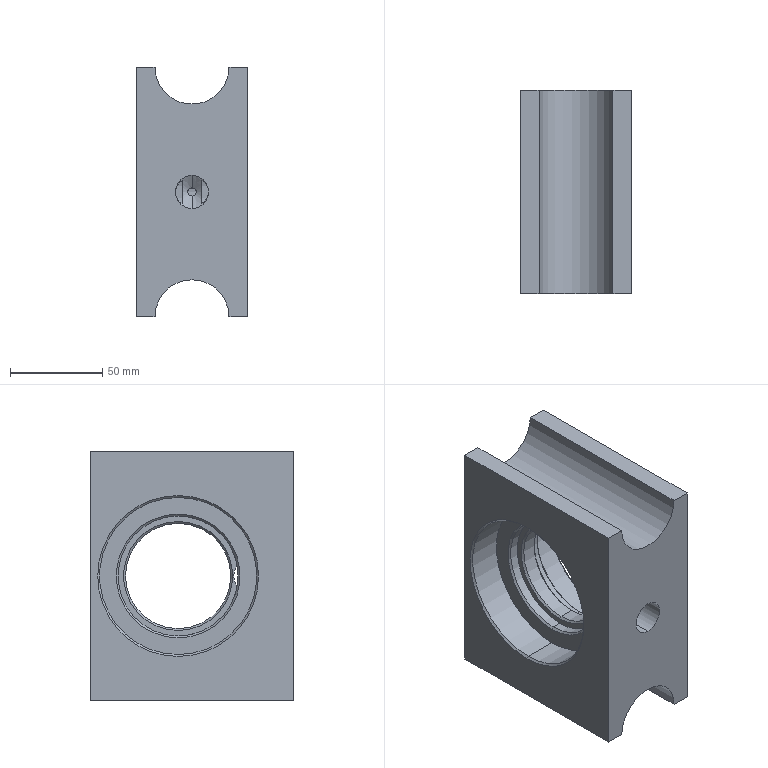Part | SolidWorks | features BaseBody 1 | 1 solid | 41 faces | box 60 x 110 x 135 mm | volume 463125 mm3 | cylinder 15 | cone 14 | plane 12 | commonest cylinder face diameters 65 x4 85 x4 40 x3 18 x2 57 x2
STEP:
#1=CARTESIAN_POINT('',(29.,7.5,42.5));
#2=VERTEX_POINT('',#1);
#3=CARTESIAN_POINT('',(29.,7.5,-42.5));
#4=VERTEX_POINT('',#3);
#5=CARTESIAN_POINT('',(29.,7.5,0.));
#6=DIRECTION('',(1.,0.,0.));
#7=DIRECTION('',(0.,0.,-1.));
#8=AXIS2_PLACEMENT_3D('',#5,#6,#7);
#9=CIRCLE('',#8,42.5);
#10=EDGE_CURVE('',#2,#4,#9,.T.);
#11=ORIENTED_EDGE('',*,*,#10,.F.);
#12=CARTESIAN_POINT('',(30.,7.5,43.5));
#13=VERTEX_POINT('',#12);
#14=CARTESIAN_POINT('',(29.,7.5,42.5));
#15=DIRECTION('',(0.7071,0.,0.7071));
#16=VECTOR('',#15,1000.);
#17=LINE('',#14,#16);
#18=EDGE_CURVE('',#2,#13,#17,.T.);
#19=ORIENTED_EDGE('',*,*,#18,.T.);
#20=CARTESIAN_POINT('',(30.,7.5,-43.5));
#21=VERTEX_POINT('',#20);
#22=CARTESIAN_POINT('',(30.,7.5,0.));
#23=DIRECTION('',(-1.,0.,0.));
#24=DIRECTION('',(0.,0.,-1.));
#25=AXIS2_PLACEMENT_3D('',#22,#23,#24);
#26=CIRCLE('',#25,43.5);
#27=EDGE_CURVE('',#21,#13,#26,.T.);
#28=ORIENTED_EDGE('',*,*,#27,.F.);
#29=CARTESIAN_POINT('',(29.,7.5,-42.5));
#30=DIRECTION('',(0.7071,0.,-0.7071));
#31=VECTOR('',#30,1000.);
#32=LINE('',#29,#31);
#33=EDGE_CURVE('',#4,#21,#32,.T.);
#34=ORIENTED_EDGE('',*,*,#33,.F.);
#35=EDGE_LOOP('',(#11,#19,#28,#34));
#36=FACE_OUTER_BOUND('',#35,.T.);
#37=CARTESIAN_POINT('',(29.,7.5,0.));
#38=DIRECTION('',(1.,0.,0.));
#39=DIRECTION('',(0.,0.,-1.));
#40=AXIS2_PLACEMENT_3D('',#37,#38,#39);
#41=CONICAL_SURFACE('',#40,42.5,0.7854);
#42=ADVANCED_FACE('',(#36),#41,.F.);
#43=CARTESIAN_POINT('',(10.,7.5,32.5));
#44=VERTEX_POINT('',#43);
#45=CARTESIAN_POINT('',(10.,7.5,-32.5));
#46=VERTEX_POINT('',#45);
#47=CARTESIAN_POINT('',(10.,7.5,0.));
#48=DIRECTION('',(1.,0.,0.));
#49=DIRECTION('',(0.,0.,-1.));
#50=AXIS2_PLACEMENT_3D('',#47,#48,#49);
#51=CIRCLE('',#50,32.5);
#52=EDGE_CURVE('',#44,#46,#51,.T.);
#53=ORIENTED_EDGE('',*,*,#52,.F.);
#54=CARTESIAN_POINT('',(11.,7.5,33.5));
#55=VERTEX_POINT('',#54);
#56=CARTESIAN_POINT('',(10.,7.5,32.5));
#57=DIRECTION('',(0.7071,0.,0.7071));
#58=VECTOR('',#57,1000.);
#59=LINE('',#56,#58);
#60=EDGE_CURVE('',#44,#55,#59,.T.);
#61=ORIENTED_EDGE('',*,*,#60,.T.);
#62=CARTESIAN_POINT('',(11.,7.5,-33.5));
#63=VERTEX_POINT('',#62);
#64=CARTESIAN_POINT('',(11.,7.5,0.));
#65=DIRECTION('',(-1.,0.,0.));
#66=DIRECTION('',(0.,0.,-1.));
#67=AXIS2_PLACEMENT_3D('',#64,#65,#66);
#68=CIRCLE('',#67,33.5);
#69=EDGE_CURVE('',#63,#55,#68,.T.);
#70=ORIENTED_EDGE('',*,*,#69,.F.);
#71=CARTESIAN_POINT('',(10.,7.5,-32.5));
#72=DIRECTION('',(0.7071,0.,-0.7071));
#73=VECTOR('',#72,1000.);
#74=LINE('',#71,#73);
#75=EDGE_CURVE('',#46,#63,#74,.T.);
#76=ORIENTED_EDGE('',*,*,#75,.F.);
#77=EDGE_LOOP('',(#53,#61,#70,#76));
#78=FACE_OUTER_BOUND('',#77,.T.);
#79=CARTESIAN_POINT('',(10.,7.5,0.));
#80=DIRECTION('',(1.,0.,0.));
#81=DIRECTION('',(0.,0.,-1.));
#82=AXIS2_PLACEMENT_3D('',#79,#80,#81);
#83=CONICAL_SURFACE('',#82,32.5,0.7854);
#84=ADVANCED_FACE('',(#78),#83,.F.);
#85=CARTESIAN_POINT('',(4.,7.5,28.5));
#86=VERTEX_POINT('',#85);
#87=CARTESIAN_POINT('',(4.,7.5,-28.5));
#88=VERTEX_POINT('',#87);
#89=CARTESIAN_POINT('',(4.,7.5,0.));
#90=DIRECTION('',(1.,0.,0.));
#91=DIRECTION('',(0.,0.,-1.));
#92=AXIS2_PLACEMENT_3D('',#89,#90,#91);
#93=CIRCLE('',#92,28.5);
#94=EDGE_CURVE('',#86,#88,#93,.T.);
#95=ORIENTED_EDGE('',*,*,#94,.F.);
#96=CARTESIAN_POINT('',(5.,7.5,29.5));
#97=VERTEX_POINT('',#96);
#98=CARTESIAN_POINT('',(4.,7.5,28.5));
#99=DIRECTION('',(0.7071,0.,0.7071));
#100=VECTOR('',#99,1000.);
#101=LINE('',#98,#100);
#102=EDGE_CURVE('',#86,#97,#101,.T.);
#103=ORIENTED_EDGE('',*,*,#102,.T.);
#104=CARTESIAN_POINT('',(5.,7.5,-29.5));
#105=VERTEX_POINT('',#104);
#106=CARTESIAN_POINT('',(5.,7.5,0.));
#107=DIRECTION('',(-1.,0.,0.));
#108=DIRECTION('',(0.,0.,-1.));
#109=AXIS2_PLACEMENT_3D('',#106,#107,#108);
#110=CIRCLE('',#109,29.5);
#111=EDGE_CURVE('',#105,#97,#110,.T.);
#112=ORIENTED_EDGE('',*,*,#111,.F.);
#113=CARTESIAN_POINT('',(4.,7.5,-28.5));
#114=DIRECTION('',(0.7071,0.,-0.7071));
#115=VECTOR('',#114,1000.);
#116=LINE('',#113,#115);
#117=EDGE_CURVE('',#88,#105,#116,.T.);
#118=ORIENTED_EDGE('',*,*,#117,.F.);
#119=EDGE_LOOP('',(#95,#103,#112,#118));
#120=FACE_OUTER_BOUND('',#119,.T.);
#121=CARTESIAN_POINT('',(4.,7.5,0.));
#122=DIRECTION('',(1.,0.,0.));
#123=DIRECTION('',(0.,0.,-1.));
#124=AXIS2_PLACEMENT_3D('',#121,#122,#123);
#125=CONICAL_SURFACE('',#124,28.5,0.7854);
#126=ADVANCED_FACE('',(#120),#125,.F.);
#127=CARTESIAN_POINT('',(-4.,7.5,-28.5));
#128=VERTEX_POINT('',#127);
#129=CARTESIAN_POINT('',(-4.,7.5,28.5));
#130=VERTEX_POINT('',#129);
#131=CARTESIAN_POINT('',(-4.,7.5,0.));
#132=DIRECTION('',(-1.,0.,0.));
#133=DIRECTION('',(0.,0.,1.));
#134=AXIS2_PLACEMENT_3D('',#131,#132,#133);
#135=CIRCLE('',#134,28.5);
#136=EDGE_CURVE('',#128,#130,#135,.T.);
#137=ORIENTED_EDGE('',*,*,#136,.F.);
#138=CARTESIAN_POINT('',(-5.,7.5,-29.5));
#139=VERTEX_POINT('',#138);
#140=CARTESIAN_POINT('',(-4.,7.5,-28.5));
#141=DIRECTION('',(-0.7071,0.,-0.7071));
#142=VECTOR('',#141,1000.);
#143=LINE('',#140,#142);
#144=EDGE_CURVE('',#128,#139,#143,.T.);
#145=ORIENTED_EDGE('',*,*,#144,.T.);
#146=CARTESIAN_POINT('',(-5.,7.5,29.5));
#147=VERTEX_POINT('',#146);
#148=CARTESIAN_POINT('',(-5.,7.5,0.));
#149=DIRECTION('',(1.,0.,0.));
#150=DIRECTION('',(0.,0.,1.));
#151=AXIS2_PLACEMENT_3D('',#148,#149,#150);
#152=CIRCLE('',#151,29.5);
#153=EDGE_CURVE('',#147,#139,#152,.T.);
#154=ORIENTED_EDGE('',*,*,#153,.F.);
#155=CARTESIAN_POINT('',(-4.,7.5,28.5));
#156=DIRECTION('',(-0.7071,0.,0.7071));
#157=VECTOR('',#156,1000.);
#158=LINE('',#155,#157);
#159=EDGE_CURVE('',#130,#147,#158,.T.);
#160=ORIENTED_EDGE('',*,*,#159,.F.);
#161=EDGE_LOOP('',(#137,#145,#154,#160));
#162=FACE_OUTER_BOUND('',#161,.T.);
#163=CARTESIAN_POINT('',(-4.,7.5,0.));
#164=DIRECTION('',(-1.,0.,0.));
#165=DIRECTION('',(0.,0.,1.));
#166=AXIS2_PLACEMENT_3D('',#163,#164,#165);
#167=CONICAL_SURFACE('',#166,28.5,0.7854);
#168=ADVANCED_FACE('',(#162),#167,.F.);
#169=CARTESIAN_POINT('',(-10.,7.5,-32.5));
#170=VERTEX_POINT('',#169);
#171=CARTESIAN_POINT('',(-10.,7.5,32.5));
#172=VERTEX_POINT('',#171);
#173=CARTESIAN_POINT('',(-10.,7.5,0.));
#174=DIRECTION('',(-1.,0.,0.));
#175=DIRECTION('',(0.,0.,1.));
#176=AXIS2_PLACEMENT_3D('',#173,#174,#175);
#177=CIRCLE('',#176,32.5);
#178=EDGE_CURVE('',#170,#172,#177,.T.);
#179=ORIENTED_EDGE('',*,*,#178,.F.);
#180=CARTESIAN_POINT('',(-11.,7.5,-33.5));
#181=VERTEX_POINT('',#180);
#182=CARTESIAN_POINT('',(-11.,7.5,-33.5));
#183=DIRECTION('',(-0.7071,0.,-0.7071));
#184=VECTOR('',#183,1000.);
#185=LINE('',#182,#184);
#186=EDGE_CURVE('',#170,#181,#185,.T.);
#187=ORIENTED_EDGE('',*,*,#186,.T.);
#188=CARTESIAN_POINT('',(-11.,7.5,33.5));
#189=VERTEX_POINT('',#188);
#190=CARTESIAN_POINT('',(-11.,7.5,0.));
#191=DIRECTION('',(1.,0.,0.));
#192=DIRECTION('',(0.,0.,1.));
#193=AXIS2_PLACEMENT_3D('',#190,#191,#192);
#194=CIRCLE('',#193,33.5);
#195=EDGE_CURVE('',#189,#181,#194,.T.);
#196=ORIENTED_EDGE('',*,*,#195,.F.);
#197=CARTESIAN_POINT('',(-11.,7.5,33.5));
#198=DIRECTION('',(-0.7071,0.,0.7071));
#199=VECTOR('',#198,1000.);
#200=LINE('',#197,#199);
#201=EDGE_CURVE('',#172,#189,#200,.T.);
#202=ORIENTED_EDGE('',*,*,#201,.F.);
#203=EDGE_LOOP('',(#179,#187,#196,#202));
#204=FACE_OUTER_BOUND('',#203,.T.);
#205=CARTESIAN_POINT('',(-11.,7.5,0.));
#206=DIRECTION('',(-1.,0.,0.));
#207=DIRECTION('',(0.,0.,1.));
#208=AXIS2_PLACEMENT_3D('',#205,#206,#207);
#209=CONICAL_SURFACE('',#208,33.5,0.7854);
#210=ADVANCED_FACE('',(#204),#209,.F.);
#211=CARTESIAN_POINT('',(-29.,7.5,-42.5));
#212=VERTEX_POINT('',#211);
#213=CARTESIAN_POINT('',(-29.,7.5,42.5));
#214=VERTEX_POINT('',#213);
#215=CARTESIAN_POINT('',(-29.,7.5,0.));
#216=DIRECTION('',(-1.,0.,0.));
#217=DIRECTION('',(0.,0.,-1.));
#218=AXIS2_PLACEMENT_3D('',#215,#216,#217);
#219=CIRCLE('',#218,42.5);
#220=EDGE_CURVE('',#212,#214,#219,.T.);
#221=ORIENTED_EDGE('',*,*,#220,.F.);
#222=CARTESIAN_POINT('',(-30.,7.5,-43.5));
#223=VERTEX_POINT('',#222);
#224=CARTESIAN_POINT('',(-30.,7.5,-43.5));
#225=DIRECTION('',(-0.7071,0.,-0.7071));
#226=VECTOR('',#225,1000.);
#227=LINE('',#224,#226);
#228=EDGE_CURVE('',#212,#223,#227,.T.);
#229=ORIENTED_EDGE('',*,*,#228,.T.);
#230=CARTESIAN_POINT('',(-30.,7.5,43.5));
#231=VERTEX_POINT('',#230);
#232=CARTESIAN_POINT('',(-30.,7.5,0.));
#233=DIRECTION('',(1.,0.,0.));
#234=DIRECTION('',(0.,0.,-1.));
#235=AXIS2_PLACEMENT_3D('',#232,#233,#234);
#236=CIRCLE('',#235,43.5);
#237=EDGE_CURVE('',#231,#223,#236,.T.);
#238=ORIENTED_EDGE('',*,*,#237,.F.);
#239=CARTESIAN_POINT('',(-30.,7.5,43.5));
#240=DIRECTION('',(-0.7071,0.,0.7071));
#241=VECTOR('',#240,1000.);
#242=LINE('',#239,#241);
#243=EDGE_CURVE('',#214,#231,#242,.T.);
#244=ORIENTED_EDGE('',*,*,#243,.F.);
#245=EDGE_LOOP('',(#221,#229,#238,#244));
#246=FACE_OUTER_BOUND('',#245,.T.);
#247=CARTESIAN_POINT('',(-30.,7.5,0.));
#248=DIRECTION('',(-1.,0.,0.));
#249=DIRECTION('',(0.,0.,1.));
#250=AXIS2_PLACEMENT_3D('',#247,#248,#249);
#251=CONICAL_SURFACE('',#250,43.5,0.7854);
#252=ADVANCED_FACE('',(#246),#251,.F.);
#253=CARTESIAN_POINT('',(-5.,-24.396,-6.238));
#254=VERTEX_POINT('',#253);
#255=CARTESIAN_POINT('',(-5.,7.5,-32.5));
#256=VERTEX_POINT('',#255);
#257=CARTESIAN_POINT('',(-5.,7.5,0.));
#258=DIRECTION('',(1.,0.,0.));
#259=DIRECTION('',(0.,0.,-1.));
#260=AXIS2_PLACEMENT_3D('',#257,#258,#259);
#261=CIRCLE('',#260,32.5);
#262=EDGE_CURVE('',#254,#256,#261,.T.);
#263=ORIENTED_EDGE('',*,*,#262,.T.);
#264=CARTESIAN_POINT('',(-5.,7.5,-32.5));
#265=DIRECTION('',(-1.,0.,0.));
#266=VECTOR('',#265,1000.);
#267=LINE('',#264,#266);
#268=EDGE_CURVE('',#256,#170,#267,.T.);
#269=ORIENTED_EDGE('',*,*,#268,.T.);
#270=ORIENTED_EDGE('',*,*,#178,.T.);
#271=CARTESIAN_POINT('',(-5.,7.5,32.5));
#272=VERTEX_POINT('',#271);
#273=CARTESIAN_POINT('',(-5.,7.5,32.5));
#274=DIRECTION('',(-1.,0.,0.));
#275=VECTOR('',#274,1000.);
#276=LINE('',#273,#275);
#277=EDGE_CURVE('',#272,#172,#276,.T.);
#278=ORIENTED_EDGE('',*,*,#277,.F.);
#279=CARTESIAN_POINT('',(-5.,-24.396,6.238));
#280=VERTEX_POINT('',#279);
#281=CARTESIAN_POINT('',(-5.,7.5,0.));
#282=DIRECTION('',(1.,0.,0.));
#283=DIRECTION('',(0.,0.,-1.));
#284=AXIS2_PLACEMENT_3D('',#281,#282,#283);
#285=CIRCLE('',#284,32.5);
#286=EDGE_CURVE('',#272,#280,#285,.T.);
#287=ORIENTED_EDGE('',*,*,#286,.T.);
#288=CARTESIAN_POINT('',(-9.,-25.,0.));
#289=VERTEX_POINT('',#288);
#290=CARTESIAN_POINT('',(-5.,-24.396,6.238));
#291=CARTESIAN_POINT('',(-5.564,-24.458,5.919));
#292=CARTESIAN_POINT('',(-6.087,-24.526,5.547));
#293=CARTESIAN_POINT('',(-6.808,-24.629,4.902));
#294=CARTESIAN_POINT('',(-7.038,-24.664,4.67));
#295=CARTESIAN_POINT('',(-7.467,-24.731,4.182));
#296=CARTESIAN_POINT('',(-7.664,-24.763,3.926));
#297=CARTESIAN_POINT('',(-8.025,-24.824,3.392));
#298=CARTESIAN_POINT('',(-8.188,-24.852,3.112));
#299=CARTESIAN_POINT('',(-8.476,-24.903,2.527));
#300=CARTESIAN_POINT('',(-8.599,-24.925,2.223));
#301=CARTESIAN_POINT('',(-8.796,-24.962,1.608));
#302=CARTESIAN_POINT('',(-8.872,-24.976,1.295));
#303=CARTESIAN_POINT('',(-8.973,-24.995,0.6557));
#304=CARTESIAN_POINT('',(-9.,-25.,0.3269));
#305=CARTESIAN_POINT('',(-9.,-25.,0.));
#306=B_SPLINE_CURVE_WITH_KNOTS('',3,(#290,#291,#292,#293,#294,#295,#296,#297,#298,#299,#300,#301,#302,#303,#304,#305),.UNSPECIFIED.,.F.,.F.,(4,2,2,2,2,2,2,4),(0.000451,0.002388,0.003357,0.004325,0.005294,0.006262,0.007231,0.008199),.UNSPECIFIED.);
#307=EDGE_CURVE('',#280,#289,#306,.T.);
#308=ORIENTED_EDGE('',*,*,#307,.T.);
#309=CARTESIAN_POINT('',(-9.,-25.,0.));
#310=CARTESIAN_POINT('',(-9.,-25.,-0.6513));
#311=CARTESIAN_POINT('',(-8.898,-24.98,-1.291));
#312=CARTESIAN_POINT('',(-8.499,-24.907,-2.535));
#313=CARTESIAN_POINT('',(-8.212,-24.855,-3.113));
#314=CARTESIAN_POINT('',(-7.485,-24.733,-4.193));
#315=CARTESIAN_POINT('',(-7.057,-24.665,-4.676));
#316=CARTESIAN_POINT('',(-6.336,-24.562,-5.325));
#317=CARTESIAN_POINT('',(-6.081,-24.527,-5.529));
#318=CARTESIAN_POINT('',(-5.555,-24.46,-5.905));
#319=CARTESIAN_POINT('',(-5.282,-24.427,-6.078));
#320=CARTESIAN_POINT('',(-5.,-24.396,-6.238));
#321=B_SPLINE_CURVE_WITH_KNOTS('',3,(#309,#310,#311,#312,#313,#314,#315,#316,#317,#318,#319,#320),.UNSPECIFIED.,.F.,.F.,(4,2,2,2,2,4),(0.008199,0.01013,0.01206,0.01399,0.01495,0.01592),.UNSPECIFIED.);
#322=EDGE_CURVE('',#289,#254,#321,.T.);
#323=ORIENTED_EDGE('',*,*,#322,.T.);
#324=EDGE_LOOP('',(#263,#269,#270,#278,#287,#308,#323));
#325=FACE_OUTER_BOUND('',#324,.T.);
#326=CARTESIAN_POINT('',(-5.,7.5,0.));
#327=DIRECTION('',(-1.,0.,0.));
#328=DIRECTION('',(0.,0.,1.));
#329=AXIS2_PLACEMENT_3D('',#326,#327,#328);
#330=CYLINDRICAL_SURFACE('',#329,32.5);
#331=ADVANCED_FACE('',(#325),#330,.F.);
#332=CARTESIAN_POINT('',(-11.,7.5,42.5));
#333=VERTEX_POINT('',#332);
#334=CARTESIAN_POINT('',(-11.,7.5,-42.5));
#335=VERTEX_POINT('',#334);
#336=CARTESIAN_POINT('',(-11.,7.5,0.));
#337=DIRECTION('',(1.,0.,0.));
#338=DIRECTION('',(0.,0.,-1.));
#339=AXIS2_PLACEMENT_3D('',#336,#337,#338);
#340=CIRCLE('',#339,42.5);
#341=EDGE_CURVE('',#333,#335,#340,.T.);
#342=ORIENTED_EDGE('',*,*,#341,.T.);
#343=CARTESIAN_POINT('',(-11.,7.5,-42.5));
#344=DIRECTION('',(-1.,0.,0.));
#345=VECTOR('',#344,1000.);
#346=LINE('',#343,#345);
#347=EDGE_CURVE('',#335,#212,#346,.T.);
#348=ORIENTED_EDGE('',*,*,#347,.T.);
#349=ORIENTED_EDGE('',*,*,#220,.T.);
#350=CARTESIAN_POINT('',(-11.,7.5,42.5));
#351=DIRECTION('',(-1.,0.,0.));
#352=VECTOR('',#351,1000.);
#353=LINE('',#350,#352);
#354=EDGE_CURVE('',#333,#214,#353,.T.);
#355=ORIENTED_EDGE('',*,*,#354,.F.);
#356=EDGE_LOOP('',(#342,#348,#349,#355));
#357=FACE_OUTER_BOUND('',#356,.T.);
#358=CARTESIAN_POINT('',(-11.,7.5,0.));
#359=DIRECTION('',(-1.,0.,0.));
#360=DIRECTION('',(0.,0.,1.));
#361=AXIS2_PLACEMENT_3D('',#358,#359,#360);
#362=CYLINDRICAL_SURFACE('',#361,42.5);
#363=ADVANCED_FACE('',(#357),#362,.F.);
#364=CARTESIAN_POINT('',(0.,-25.,9.));
#365=VERTEX_POINT('',#364);
#366=CARTESIAN_POINT('',(0.,-25.,0.));
#367=DIRECTION('',(0.,-1.,0.));
#368=DIRECTION('',(0.,0.,-1.));
#369=AXIS2_PLACEMENT_3D('',#366,#367,#368);
#370=CIRCLE('',#369,9.);
#371=EDGE_CURVE('',#365,#289,#370,.T.);
#372=ORIENTED_EDGE('',*,*,#371,.F.);
#373=CARTESIAN_POINT('',(0.,-55.,9.));
#374=VERTEX_POINT('',#373);
#375=CARTESIAN_POINT('',(0.,-55.,9.));
#376=DIRECTION('',(0.,-1.,0.));
#377=VECTOR('',#376,1000.);
#378=LINE('',#375,#377);
#379=EDGE_CURVE('',#365,#374,#378,.T.);
#380=ORIENTED_EDGE('',*,*,#379,.T.);
#381=CARTESIAN_POINT('',(0.,-55.,-9.));
#382=VERTEX_POINT('',#381);
#383=CARTESIAN_POINT('',(0.,-55.,0.));
#384=DIRECTION('',(0.,-1.,0.));
#385=DIRECTION('',(0.,0.,-1.));
#386=AXIS2_PLACEMENT_3D('',#383,#384,#385);
#387=CIRCLE('',#386,9.);
#388=EDGE_CURVE('',#374,#382,#387,.T.);
#389=ORIENTED_EDGE('',*,*,#388,.T.);
#390=CARTESIAN_POINT('',(0.,-25.,-9.));
#391=VERTEX_POINT('',#390);
#392=CARTESIAN_POINT('',(0.,-55.,-9.));
#393=DIRECTION('',(0.,-1.,0.));
#394=VECTOR('',#393,1000.);
#395=LINE('',#392,#394);
#396=EDGE_CURVE('',#391,#382,#395,.T.);
#397=ORIENTED_EDGE('',*,*,#396,.F.);
#398=CARTESIAN_POINT('',(0.,-25.,0.));
#399=DIRECTION('',(0.,-1.,0.));
#400=DIRECTION('',(0.,0.,-1.));
#401=AXIS2_PLACEMENT_3D('',#398,#399,#400);
#402=CIRCLE('',#401,9.);
#403=EDGE_CURVE('',#289,#391,#402,.T.);
#404=ORIENTED_EDGE('',*,*,#403,.F.);
#405=EDGE_LOOP('',(#372,#380,#389,#397,#404));
#406=FACE_OUTER_BOUND('',#405,.T.);
#407=CARTESIAN_POINT('',(0.,-55.,0.));
#408=DIRECTION('',(0.,-1.,0.));
#409=DIRECTION('',(0.,0.,-1.));
#410=AXIS2_PLACEMENT_3D('',#407,#408,#409);
#411=CYLINDRICAL_SURFACE('',#410,9.);
#412=ADVANCED_FACE('',(#406),#411,.F.);
#413=CARTESIAN_POINT('',(0.,-55.,-47.5));
#414=VERTEX_POINT('',#413);
#415=CARTESIAN_POINT('',(20.,-55.,-67.5));
#416=VERTEX_POINT('',#415);
#417=CARTESIAN_POINT('',(0.,-55.,-67.5));
#418=DIRECTION('',(0.,1.,0.));
#419=DIRECTION('',(0.,0.,1.));
#420=AXIS2_PLACEMENT_3D('',#417,#418,#419);
#421=CIRCLE('',#420,20.);
#422=EDGE_CURVE('',#414,#416,#421,.T.);
#423=ORIENTED_EDGE('',*,*,#422,.F.);
#424=CARTESIAN_POINT('',(0.,55.,-47.5));
#425=VERTEX_POINT('',#424);
#426=CARTESIAN_POINT('',(0.,-55.,-47.5));
#427=DIRECTION('',(0.,1.,0.));
#428=VECTOR('',#427,1000.);
#429=LINE('',#426,#428);
#430=EDGE_CURVE('',#414,#425,#429,.T.);
#431=ORIENTED_EDGE('',*,*,#430,.T.);
#432=CARTESIAN_POINT('',(20.,55.,-67.5));
#433=VERTEX_POINT('',#432);
#434=CARTESIAN_POINT('',(0.,55.,-67.5));
#435=DIRECTION('',(0.,1.,0.));
#436=DIRECTION('',(0.,0.,1.));
#437=AXIS2_PLACEMENT_3D('',#434,#435,#436);
#438=CIRCLE('',#437,20.);
#439=EDGE_CURVE('',#425,#433,#438,.T.);
#440=ORIENTED_EDGE('',*,*,#439,.T.);
#441=CARTESIAN_POINT('',(20.,-55.,-67.5));
#442=DIRECTION('',(0.,1.,0.));
#443=VECTOR('',#442,1000.);
#444=LINE('',#441,#443);
#445=EDGE_CURVE('',#416,#433,#444,.T.);
#446=ORIENTED_EDGE('',*,*,#445,.F.);
#447=EDGE_LOOP('',(#423,#431,#440,#446));
#448=FACE_OUTER_BOUND('',#447,.T.);
#449=CARTESIAN_POINT('',(0.,-55.,-67.5));
#450=DIRECTION('',(0.,1.,0.));
#451=DIRECTION('',(0.,0.,1.));
#452=AXIS2_PLACEMENT_3D('',#449,#450,#451);
#453=CYLINDRICAL_SURFACE('',#452,20.);
#454=ADVANCED_FACE('',(#448),#453,.F.);
#455=CARTESIAN_POINT('',(5.,7.5,32.5));
#456=VERTEX_POINT('',#455);
#457=CARTESIAN_POINT('',(5.,-24.396,6.238));
#458=VERTEX_POINT('',#457);
#459=CARTESIAN_POINT('',(5.,7.5,0.));
#460=DIRECTION('',(1.,0.,0.));
#461=DIRECTION('',(0.,0.,-1.));
#462=AXIS2_PLACEMENT_3D('',#459,#460,#461);
#463=CIRCLE('',#462,32.5);
#464=EDGE_CURVE('',#456,#458,#463,.T.);
#465=ORIENTED_EDGE('',*,*,#464,.F.);
#466=CARTESIAN_POINT('',(5.,7.5,32.5));
#467=DIRECTION('',(1.,0.,0.));
#468=VECTOR('',#467,1000.);
#469=LINE('',#466,#468);
#470=EDGE_CURVE('',#456,#44,#469,.T.);
#471=ORIENTED_EDGE('',*,*,#470,.T.);
#472=ORIENTED_EDGE('',*,*,#52,.T.);
#473=CARTESIAN_POINT('',(5.,7.5,-32.5));
#474=VERTEX_POINT('',#473);
#475=CARTESIAN_POINT('',(5.,7.5,-32.5));
#476=DIRECTION('',(1.,0.,0.));
#477=VECTOR('',#476,1000.);
#478=LINE('',#475,#477);
#479=EDGE_CURVE('',#474,#46,#478,.T.);
#480=ORIENTED_EDGE('',*,*,#479,.F.);
#481=CARTESIAN_POINT('',(5.,-24.396,-6.238));
#482=VERTEX_POINT('',#481);
#483=CARTESIAN_POINT('',(5.,7.5,0.));
#484=DIRECTION('',(1.,0.,0.));
#485=DIRECTION('',(0.,0.,-1.));
#486=AXIS2_PLACEMENT_3D('',#483,#484,#485);
#487=CIRCLE('',#486,32.5);
#488=EDGE_CURVE('',#482,#474,#487,.T.);
#489=ORIENTED_EDGE('',*,*,#488,.F.);
#490=CARTESIAN_POINT('',(9.,-25.,0.));
#491=VERTEX_POINT('',#490);
#492=CARTESIAN_POINT('',(5.,-24.396,-6.238));
#493=CARTESIAN_POINT('',(5.564,-24.458,-5.919));
#494=CARTESIAN_POINT('',(6.087,-24.526,-5.547));
#495=CARTESIAN_POINT('',(6.808,-24.629,-4.902));
#496=CARTESIAN_POINT('',(7.038,-24.664,-4.67));
#497=CARTESIAN_POINT('',(7.467,-24.731,-4.182));
#498=CARTESIAN_POINT('',(7.664,-24.763,-3.926));
#499=CARTESIAN_POINT('',(8.025,-24.824,-3.392));
#500=CARTESIAN_POINT('',(8.188,-24.852,-3.112));
#501=CARTESIAN_POINT('',(8.476,-24.903,-2.527));
#502=CARTESIAN_POINT('',(8.599,-24.925,-2.223));
#503=CARTESIAN_POINT('',(8.796,-24.962,-1.608));
#504=CARTESIAN_POINT('',(8.872,-24.976,-1.295));
#505=CARTESIAN_POINT('',(8.973,-24.995,-0.6557));
#506=CARTESIAN_POINT('',(9.,-25.,-0.3269));
#507=CARTESIAN_POINT('',(9.,-25.,0.));
#508=B_SPLINE_CURVE_WITH_KNOTS('',3,(#492,#493,#494,#495,#496,#497,#498,#499,#500,#501,#502,#503,#504,#505,#506,#507),.UNSPECIFIED.,.F.,.F.,(4,2,2,2,2,2,2,4),(0.000451,0.002388,0.003357,0.004325,0.005294,0.006262,0.007231,0.008199),.UNSPECIFIED.);
#509=EDGE_CURVE('',#482,#491,#508,.T.);
#510=ORIENTED_EDGE('',*,*,#509,.T.);
#511=CARTESIAN_POINT('',(9.,-25.,0.));
#512=CARTESIAN_POINT('',(9.,-25.,0.6513));
#513=CARTESIAN_POINT('',(8.898,-24.98,1.291));
#514=CARTESIAN_POINT('',(8.499,-24.907,2.535));
#515=CARTESIAN_POINT('',(8.212,-24.855,3.113));
#516=CARTESIAN_POINT('',(7.485,-24.733,4.193));
#517=CARTESIAN_POINT('',(7.057,-24.665,4.676));
#518=CARTESIAN_POINT('',(6.336,-24.562,5.325));
#519=CARTESIAN_POINT('',(6.081,-24.527,5.529));
#520=CARTESIAN_POINT('',(5.555,-24.46,5.905));
#521=CARTESIAN_POINT('',(5.282,-24.427,6.078));
#522=CARTESIAN_POINT('',(5.,-24.396,6.238));
#523=B_SPLINE_CURVE_WITH_KNOTS('',3,(#511,#512,#513,#514,#515,#516,#517,#518,#519,#520,#521,#522),.UNSPECIFIED.,.F.,.F.,(4,2,2,2,2,4),(0.008199,0.01013,0.01206,0.01399,0.01495,0.01592),.UNSPECIFIED.);
#524=EDGE_CURVE('',#491,#458,#523,.T.);
#525=ORIENTED_EDGE('',*,*,#524,.T.);
#526=EDGE_LOOP('',(#465,#471,#472,#480,#489,#510,#525));
#527=FACE_OUTER_BOUND('',#526,.T.);
#528=CARTESIAN_POINT('',(5.,7.5,0.));
#529=DIRECTION('',(1.,0.,0.));
#530=DIRECTION('',(0.,0.,-1.));
#531=AXIS2_PLACEMENT_3D('',#528,#529,#530);
#532=CYLINDRICAL_SURFACE('',#531,32.5);
#533=ADVANCED_FACE('',(#527),#532,.F.);
#534=CARTESIAN_POINT('',(11.,7.5,42.5));
#535=VERTEX_POINT('',#534);
#536=CARTESIAN_POINT('',(11.,7.5,-42.5));
#537=VERTEX_POINT('',#536);
#538=CARTESIAN_POINT('',(11.,7.5,0.));
#539=DIRECTION('',(1.,0.,0.));
#540=DIRECTION('',(0.,0.,-1.));
#541=AXIS2_PLACEMENT_3D('',#538,#539,#540);
#542=CIRCLE('',#541,42.5);
#543=EDGE_CURVE('',#535,#537,#542,.T.);
#544=ORIENTED_EDGE('',*,*,#543,.F.);
#545=CARTESIAN_POINT('',(11.,7.5,42.5));
#546=DIRECTION('',(1.,0.,0.));
#547=VECTOR('',#546,1000.);
#548=LINE('',#545,#547);
#549=EDGE_CURVE('',#535,#2,#548,.T.);
#550=ORIENTED_EDGE('',*,*,#549,.T.);
#551=ORIENTED_EDGE('',*,*,#10,.T.);
#552=CARTESIAN_POINT('',(11.,7.5,-42.5));
#553=DIRECTION('',(1.,0.,0.));
#554=VECTOR('',#553,1000.);
#555=LINE('',#552,#554);
#556=EDGE_CURVE('',#537,#4,#555,.T.);
#557=ORIENTED_EDGE('',*,*,#556,.F.);
#558=EDGE_LOOP('',(#544,#550,#551,#557));
#559=FACE_OUTER_BOUND('',#558,.T.);
#560=CARTESIAN_POINT('',(11.,7.5,0.));
#561=DIRECTION('',(1.,0.,0.));
#562=DIRECTION('',(0.,0.,-1.));
#563=AXIS2_PLACEMENT_3D('',#560,#561,#562);
#564=CYLINDRICAL_SURFACE('',#563,42.5);
#565=ADVANCED_FACE('',(#559),#564,.F.);
#566=CARTESIAN_POINT('',(0.,-20.915,-2.201));
#567=VERTEX_POINT('',#566);
#568=CARTESIAN_POINT('',(0.,-20.915,2.201));
#569=VERTEX_POINT('',#568);
#570=CARTESIAN_POINT('',(0.,-20.915,-2.201));
#571=CARTESIAN_POINT('',(-0.1492,-20.915,-2.201));
#572=CARTESIAN_POINT('',(-0.2967,-20.916,-2.188));
#573=CARTESIAN_POINT('',(-0.5881,-20.92,-2.135));
#574=CARTESIAN_POINT('',(-0.7336,-20.923,-2.095));
#575=CARTESIAN_POINT('',(-1.012,-20.931,-1.99));
#576=CARTESIAN_POINT('',(-1.145,-20.935,-1.925));
#577=CARTESIAN_POINT('',(-1.398,-20.945,-1.771));
#578=CARTESIAN_POINT('',(-1.519,-20.951,-1.681));
#579=CARTESIAN_POINT('',(-1.849,-20.967,-1.381));
#580=CARTESIAN_POINT('',(-2.03,-20.979,-1.136));
#581=CARTESIAN_POINT('',(-2.215,-20.991,-0.73));
#582=CARTESIAN_POINT('',(-2.263,-20.994,-0.5864));
#583=CARTESIAN_POINT('',(-2.327,-20.999,-0.2971));
#584=CARTESIAN_POINT('',(-2.343,-21.,-0.1498));
#585=CARTESIAN_POINT('',(-2.343,-21.,0.1499));
#586=CARTESIAN_POINT('',(-2.327,-20.999,0.2982));
#587=CARTESIAN_POINT('',(-2.263,-20.994,0.5876));
#588=CARTESIAN_POINT('',(-2.215,-20.991,0.731));
#589=CARTESIAN_POINT('',(-2.091,-20.983,1.002));
#590=CARTESIAN_POINT('',(-2.016,-20.978,1.129));
#591=CARTESIAN_POINT('',(-1.839,-20.967,1.37));
#592=CARTESIAN_POINT('',(-1.739,-20.962,1.481));
#593=CARTESIAN_POINT('',(-1.52,-20.951,1.68));
#594=CARTESIAN_POINT('',(-1.399,-20.945,1.77));
#595=CARTESIAN_POINT('',(-1.145,-20.935,1.925));
#596=CARTESIAN_POINT('',(-1.011,-20.93,1.99));
#597=CARTESIAN_POINT('',(-0.7338,-20.923,2.095));
#598=CARTESIAN_POINT('',(-0.5883,-20.92,2.135));
#599=CARTESIAN_POINT('',(-0.296,-20.916,2.188));
#600=CARTESIAN_POINT('',(-0.1487,-20.915,2.201));
#601=CARTESIAN_POINT('',(0.,-20.915,2.201));
#602=B_SPLINE_CURVE_WITH_KNOTS('',3,(#570,#571,#572,#573,#574,#575,#576,#577,#578,#579,#580,#581,#582,#583,#584,#585,#586,#587,#588,#589,#590,#591,#592,#593,#594,#595,#596,#597,#598,#599,#600,#601),.UNSPECIFIED.,.F.,.F.,(4,2,2,2,2,2,2,2,2,2,2,2,2,2,2,4),(0.01202,0.01247,0.01291,0.01336,0.01381,0.0147,0.01514,0.01559,0.01603,0.01648,0.01693,0.01737,0.01782,0.01826,0.01871,0.01915),.UNSPECIFIED.);
#603=EDGE_CURVE('',#567,#569,#602,.T.);
#604=ORIENTED_EDGE('',*,*,#603,.T.);
#605=CARTESIAN_POINT('',(0.,-25.,9.));
#606=DIRECTION('',(0.,-0.515,0.8572));
#607=VECTOR('',#606,1000.);
#608=LINE('',#605,#607);
#609=EDGE_CURVE('',#569,#365,#608,.T.);
#610=ORIENTED_EDGE('',*,*,#609,.T.);
#611=ORIENTED_EDGE('',*,*,#371,.T.);
#612=ORIENTED_EDGE('',*,*,#307,.F.);
#613=CARTESIAN_POINT('',(-5.,-24.396,-6.238));
#614=CARTESIAN_POINT('',(-5.,-24.164,-5.743));
#615=CARTESIAN_POINT('',(-5.,-23.94,-5.244));
#616=CARTESIAN_POINT('',(-5.,-23.524,-4.236));
#617=CARTESIAN_POINT('',(-5.,-23.33,-3.726));
#618=CARTESIAN_POINT('',(-5.,-22.993,-2.687));
#619=CARTESIAN_POINT('',(-5.,-22.849,-2.154));
#620=CARTESIAN_POINT('',(-5.,-22.651,-1.082));
#621=CARTESIAN_POINT('',(-5.,-22.596,-0.5424));
#622=CARTESIAN_POINT('',(-5.,-22.597,0.5453));
#623=CARTESIAN_POINT('',(-5.,-22.653,1.098));
#624=CARTESIAN_POINT('',(-5.,-22.853,2.17));
#625=CARTESIAN_POINT('',(-5.,-22.995,2.694));
#626=CARTESIAN_POINT('',(-5.,-23.33,3.727));
#627=CARTESIAN_POINT('',(-5.,-23.524,4.237));
#628=CARTESIAN_POINT('',(-5.,-23.941,5.246));
#629=CARTESIAN_POINT('',(-5.,-24.164,5.744));
#630=CARTESIAN_POINT('',(-5.,-24.396,6.238));
#631=B_SPLINE_CURVE_WITH_KNOTS('',3,(#613,#614,#615,#616,#617,#618,#619,#620,#621,#622,#623,#624,#625,#626,#627,#628,#629,#630),.UNSPECIFIED.,.F.,.F.,(4,2,2,2,2,2,2,2,4),(0.02441,0.02605,0.02769,0.02933,0.03096,0.0326,0.03424,0.03588,0.03752),.UNSPECIFIED.);
#632=EDGE_CURVE('',#254,#280,#631,.T.);
#633=ORIENTED_EDGE('',*,*,#632,.F.);
#634=ORIENTED_EDGE('',*,*,#322,.F.);
#635=ORIENTED_EDGE('',*,*,#403,.T.);
#636=CARTESIAN_POINT('',(0.,-25.,-9.));
#637=DIRECTION('',(0.,-0.515,-0.8572));
#638=VECTOR('',#637,1000.);
#639=LINE('',#636,#638);
#640=EDGE_CURVE('',#567,#391,#639,.T.);
#641=ORIENTED_EDGE('',*,*,#640,.F.);
#642=EDGE_LOOP('',(#604,#610,#611,#612,#633,#634,#635,#641));
#643=FACE_OUTER_BOUND('',#642,.T.);
#644=CARTESIAN_POINT('',(0.,-25.,0.));
#645=DIRECTION('',(0.,-1.,0.));
#646=DIRECTION('',(0.,0.,-1.));
#647=AXIS2_PLACEMENT_3D('',#644,#645,#646);
#648=CONICAL_SURFACE('',#647,9.,1.03);
#649=ADVANCED_FACE('',(#643),#648,.F.);
#650=ORIENTED_EDGE('',*,*,#603,.F.);
#651=CARTESIAN_POINT('',(0.,-20.915,2.201));
#652=CARTESIAN_POINT('',(0.1487,-20.915,2.201));
#653=CARTESIAN_POINT('',(0.299,-20.916,2.188));
#654=CARTESIAN_POINT('',(0.5904,-20.92,2.134));
#655=CARTESIAN_POINT('',(0.733,-20.923,2.095));
#656=CARTESIAN_POINT('',(1.012,-20.931,1.99));
#657=CARTESIAN_POINT('',(1.147,-20.935,1.924));
#658=CARTESIAN_POINT('',(1.399,-20.945,1.77));
#659=CARTESIAN_POINT('',(1.518,-20.951,1.682));
#660=CARTESIAN_POINT('',(1.85,-20.967,1.38));
#661=CARTESIAN_POINT('',(2.028,-20.979,1.139));
#662=CARTESIAN_POINT('',(2.215,-20.991,0.7311));
#663=CARTESIAN_POINT('',(2.262,-20.994,0.5907));
#664=CARTESIAN_POINT('',(2.326,-20.999,0.3015));
#665=CARTESIAN_POINT('',(2.343,-21.,0.1508));
#666=CARTESIAN_POINT('',(2.343,-21.,-0.1464));
#667=CARTESIAN_POINT('',(2.327,-20.999,-0.2937));
#668=CARTESIAN_POINT('',(2.264,-20.994,-0.5859));
#669=CARTESIAN_POINT('',(2.216,-20.991,-0.7282));
#670=CARTESIAN_POINT('',(2.093,-20.983,-0.9981));
#671=CARTESIAN_POINT('',(2.017,-20.978,-1.128));
#672=CARTESIAN_POINT('',(1.841,-20.967,-1.368));
#673=CARTESIAN_POINT('',(1.741,-20.962,-1.478));
#674=CARTESIAN_POINT('',(1.521,-20.951,-1.679));
#675=CARTESIAN_POINT('',(1.4,-20.945,-1.769));
#676=CARTESIAN_POINT('',(1.147,-20.935,-1.924));
#677=CARTESIAN_POINT('',(1.014,-20.931,-1.989));
#678=CARTESIAN_POINT('',(0.7334,-20.923,-2.095));
#679=CARTESIAN_POINT('',(0.5903,-20.92,-2.135));
#680=CARTESIAN_POINT('',(0.2988,-20.916,-2.188));
#681=CARTESIAN_POINT('',(0.1493,-20.915,-2.201));
#682=CARTESIAN_POINT('',(0.,-20.915,-2.201));
#683=B_SPLINE_CURVE_WITH_KNOTS('',3,(#651,#652,#653,#654,#655,#656,#657,#658,#659,#660,#661,#662,#663,#664,#665,#666,#667,#668,#669,#670,#671,#672,#673,#674,#675,#676,#677,#678,#679,#680,#681,#682),.UNSPECIFIED.,.F.,.F.,(4,2,2,2,2,2,2,2,2,2,2,2,2,2,2,4),(0.004889,0.005335,0.005781,0.006227,0.006673,0.007565,0.00801,0.008456,0.008902,0.009348,0.009794,0.01024,0.01069,0.01113,0.01158,0.01202),.UNSPECIFIED.);
#684=EDGE_CURVE('',#569,#567,#683,.T.);
#685=ORIENTED_EDGE('',*,*,#684,.F.);
#686=EDGE_LOOP('',(#650,#685));
#687=FACE_BOUND('',#686,.T.);
#688=ORIENTED_EDGE('',*,*,#94,.T.);
#689=CARTESIAN_POINT('',(30.,7.5,-28.5));
#690=DIRECTION('',(-1.,0.,0.));
#691=VECTOR('',#690,1000.);
#692=LINE('',#689,#691);
#693=EDGE_CURVE('',#88,#128,#692,.T.);
#694=ORIENTED_EDGE('',*,*,#693,.T.);
#695=ORIENTED_EDGE('',*,*,#136,.T.);
#696=CARTESIAN_POINT('',(30.,7.5,28.5));
#697=DIRECTION('',(-1.,0.,0.));
#698=VECTOR('',#697,1000.);
#699=LINE('',#696,#698);
#700=EDGE_CURVE('',#86,#130,#699,.T.);
#701=ORIENTED_EDGE('',*,*,#700,.F.);
#702=EDGE_LOOP('',(#688,#694,#695,#701));
#703=FACE_OUTER_BOUND('',#702,.T.);
#704=CARTESIAN_POINT('',(30.,7.5,0.));
#705=DIRECTION('',(-1.,0.,0.));
#706=DIRECTION('',(0.,0.,1.));
#707=AXIS2_PLACEMENT_3D('',#704,#705,#706);
#708=CYLINDRICAL_SURFACE('',#707,28.5);
#709=ADVANCED_FACE('',(#687,#703),#708,.F.);
#710=ORIENTED_EDGE('',*,*,#693,.F.);
#711=CARTESIAN_POINT('',(4.,7.5,0.));
#712=DIRECTION('',(1.,0.,0.));
#713=DIRECTION('',(0.,0.,-1.));
#714=AXIS2_PLACEMENT_3D('',#711,#712,#713);
#715=CIRCLE('',#714,28.5);
#716=EDGE_CURVE('',#88,#86,#715,.T.);
#717=ORIENTED_EDGE('',*,*,#716,.T.);
#718=ORIENTED_EDGE('',*,*,#700,.T.);
#719=CARTESIAN_POINT('',(-4.,7.5,0.));
#720=DIRECTION('',(-1.,0.,0.));
#721=DIRECTION('',(0.,0.,1.));
#722=AXIS2_PLACEMENT_3D('',#719,#720,#721);
#723=CIRCLE('',#722,28.5);
#724=EDGE_CURVE('',#130,#128,#723,.T.);
#725=ORIENTED_EDGE('',*,*,#724,.T.);
#726=EDGE_LOOP('',(#710,#717,#718,#725));
#727=FACE_OUTER_BOUND('',#726,.T.);
#728=CARTESIAN_POINT('',(30.,7.5,0.));
#729=DIRECTION('',(-1.,0.,0.));
#730=DIRECTION('',(0.,0.,1.));
#731=AXIS2_PLACEMENT_3D('',#728,#729,#730);
#732=CYLINDRICAL_SURFACE('',#731,28.5);
#733=ADVANCED_FACE('',(#727),#732,.F.);
#734=ORIENTED_EDGE('',*,*,#609,.F.);
#735=ORIENTED_EDGE('',*,*,#684,.T.);
#736=ORIENTED_EDGE('',*,*,#640,.T.);
#737=CARTESIAN_POINT('',(0.,-25.,0.));
#738=DIRECTION('',(0.,-1.,0.));
#739=DIRECTION('',(0.,0.,-1.));
#740=AXIS2_PLACEMENT_3D('',#737,#738,#739);
#741=CIRCLE('',#740,9.);
#742=EDGE_CURVE('',#391,#491,#741,.T.);
#743=ORIENTED_EDGE('',*,*,#742,.T.);
#744=ORIENTED_EDGE('',*,*,#509,.F.);
#745=CARTESIAN_POINT('',(5.,-24.396,-6.238));
#746=CARTESIAN_POINT('',(5.,-24.164,-5.744));
#747=CARTESIAN_POINT('',(5.,-23.941,-5.246));
#748=CARTESIAN_POINT('',(5.,-23.524,-4.238));
#749=CARTESIAN_POINT('',(5.,-23.331,-3.728));
#750=CARTESIAN_POINT('',(5.,-22.993,-2.688));
#751=CARTESIAN_POINT('',(5.,-22.85,-2.157));
#752=CARTESIAN_POINT('',(5.,-22.652,-1.09));
#753=CARTESIAN_POINT('',(5.,-22.597,-0.5502));
#754=CARTESIAN_POINT('',(5.,-22.596,0.2697));
#755=CARTESIAN_POINT('',(5.,-22.61,0.5461));
#756=CARTESIAN_POINT('',(5.,-22.663,1.091));
#757=CARTESIAN_POINT('',(5.,-22.702,1.361));
#758=CARTESIAN_POINT('',(5.,-22.852,2.164));
#759=CARTESIAN_POINT('',(5.,-22.994,2.69));
#760=CARTESIAN_POINT('',(5.,-23.331,3.73));
#761=CARTESIAN_POINT('',(5.,-23.526,4.243));
#762=CARTESIAN_POINT('',(5.,-23.943,5.25));
#763=CARTESIAN_POINT('',(5.,-24.165,5.746));
#764=CARTESIAN_POINT('',(5.,-24.396,6.238));
#765=B_SPLINE_CURVE_WITH_KNOTS('',3,(#745,#746,#747,#748,#749,#750,#751,#752,#753,#754,#755,#756,#757,#758,#759,#760,#761,#762,#763,#764),.UNSPECIFIED.,.F.,.F.,(4,2,2,2,2,2,2,2,2,4),(0.04684,0.04848,0.05012,0.05175,0.05339,0.0542,0.05502,0.05666,0.05829,0.05993),.UNSPECIFIED.);
#766=EDGE_CURVE('',#482,#458,#765,.T.);
#767=ORIENTED_EDGE('',*,*,#766,.T.);
#768=ORIENTED_EDGE('',*,*,#524,.F.);
#769=CARTESIAN_POINT('',(0.,-25.,0.));
#770=DIRECTION('',(0.,-1.,0.));
#771=DIRECTION('',(0.,0.,-1.));
#772=AXIS2_PLACEMENT_3D('',#769,#770,#771);
#773=CIRCLE('',#772,9.);
#774=EDGE_CURVE('',#491,#365,#773,.T.);
#775=ORIENTED_EDGE('',*,*,#774,.T.);
#776=EDGE_LOOP('',(#734,#735,#736,#743,#744,#767,#768,#775));
#777=FACE_OUTER_BOUND('',#776,.T.);
#778=CARTESIAN_POINT('',(0.,-25.,0.));
#779=DIRECTION('',(0.,-1.,0.));
#780=DIRECTION('',(0.,0.,-1.));
#781=AXIS2_PLACEMENT_3D('',#778,#779,#780);
#782=CONICAL_SURFACE('',#781,9.,1.03);
#783=ADVANCED_FACE('',(#777),#782,.F.);
#784=CARTESIAN_POINT('',(30.,-55.,-67.5));
#785=VERTEX_POINT('',#784);
#786=CARTESIAN_POINT('',(30.,-55.,-67.5));
#787=DIRECTION('',(-1.,0.,0.));
#788=VECTOR('',#787,1000.);
#789=LINE('',#786,#788);
#790=EDGE_CURVE('',#785,#416,#789,.T.);
#791=ORIENTED_EDGE('',*,*,#790,.T.);
#792=ORIENTED_EDGE('',*,*,#445,.T.);
#793=CARTESIAN_POINT('',(30.,55.,-67.5));
#794=VERTEX_POINT('',#793);
#795=CARTESIAN_POINT('',(30.,55.,-67.5));
#796=DIRECTION('',(-1.,0.,0.));
#797=VECTOR('',#796,1000.);
#798=LINE('',#795,#797);
#799=EDGE_CURVE('',#794,#433,#798,.T.);
#800=ORIENTED_EDGE('',*,*,#799,.F.);
#801=CARTESIAN_POINT('',(30.,55.,-67.5));
#802=DIRECTION('',(0.,1.,0.));
#803=VECTOR('',#802,1000.);
#804=LINE('',#801,#803);
#805=EDGE_CURVE('',#785,#794,#804,.T.);
#806=ORIENTED_EDGE('',*,*,#805,.F.);
#807=EDGE_LOOP('',(#791,#792,#800,#806));
#808=FACE_OUTER_BOUND('',#807,.T.);
#809=CARTESIAN_POINT('',(30.,55.,-67.5));
#810=DIRECTION('',(0.,0.,1.));
#811=DIRECTION('',(0.,-1.,0.));
#812=AXIS2_PLACEMENT_3D('',#809,#810,#811);
#813=PLANE('',#812);
#814=ADVANCED_FACE('',(#808),#813,.F.);
#815=CARTESIAN_POINT('',(-20.,-55.,67.5));
#816=VERTEX_POINT('',#815);
#817=CARTESIAN_POINT('',(-30.,-55.,67.5));
#818=VERTEX_POINT('',#817);
#819=CARTESIAN_POINT('',(30.,-55.,67.5));
#820=DIRECTION('',(-1.,0.,0.));
#821=VECTOR('',#820,1000.);
#822=LINE('',#819,#821);
#823=EDGE_CURVE('',#816,#818,#822,.T.);
#824=ORIENTED_EDGE('',*,*,#823,.F.);
#825=CARTESIAN_POINT('',(-20.,55.,67.5));
#826=VERTEX_POINT('',#825);
#827=CARTESIAN_POINT('',(-20.,-55.,67.5));
#828=DIRECTION('',(0.,1.,0.));
#829=VECTOR('',#828,1000.);
#830=LINE('',#827,#829);
#831=EDGE_CURVE('',#816,#826,#830,.T.);
#832=ORIENTED_EDGE('',*,*,#831,.T.);
#833=CARTESIAN_POINT('',(-30.,55.,67.5));
#834=VERTEX_POINT('',#833);
#835=CARTESIAN_POINT('',(30.,55.,67.5));
#836=DIRECTION('',(-1.,0.,0.));
#837=VECTOR('',#836,1000.);
#838=LINE('',#835,#837);
#839=EDGE_CURVE('',#826,#834,#838,.T.);
#840=ORIENTED_EDGE('',*,*,#839,.T.);
#841=CARTESIAN_POINT('',(-30.,55.,67.5));
#842=DIRECTION('',(0.,-1.,0.));
#843=VECTOR('',#842,1000.);
#844=LINE('',#841,#843);
#845=EDGE_CURVE('',#834,#818,#844,.T.);
#846=ORIENTED_EDGE('',*,*,#845,.T.);
#847=EDGE_LOOP('',(#824,#832,#840,#846));
#848=FACE_OUTER_BOUND('',#847,.T.);
#849=CARTESIAN_POINT('',(30.,55.,67.5));
#850=DIRECTION('',(0.,0.,-1.));
#851=DIRECTION('',(0.,1.,0.));
#852=AXIS2_PLACEMENT_3D('',#849,#850,#851);
#853=PLANE('',#852);
#854=ADVANCED_FACE('',(#848),#853,.F.);
#855=ORIENTED_EDGE('',*,*,#27,.T.);
#856=CARTESIAN_POINT('',(30.,7.5,0.));
#857=DIRECTION('',(-1.,0.,0.));
#858=DIRECTION('',(0.,0.,-1.));
#859=AXIS2_PLACEMENT_3D('',#856,#857,#858);
#860=CIRCLE('',#859,43.5);
#861=EDGE_CURVE('',#13,#21,#860,.T.);
#862=ORIENTED_EDGE('',*,*,#861,.T.);
#863=EDGE_LOOP('',(#855,#862));
#864=FACE_BOUND('',#863,.T.);
#865=ORIENTED_EDGE('',*,*,#805,.T.);
#866=CARTESIAN_POINT('',(30.,55.,67.5));
#867=VERTEX_POINT('',#866);
#868=CARTESIAN_POINT('',(30.,55.,67.5));
#869=DIRECTION('',(0.,0.,1.));
#870=VECTOR('',#869,1000.);
#871=LINE('',#868,#870);
#872=EDGE_CURVE('',#794,#867,#871,.T.);
#873=ORIENTED_EDGE('',*,*,#872,.T.);
#874=CARTESIAN_POINT('',(30.,-55.,67.5));
#875=VERTEX_POINT('',#874);
#876=CARTESIAN_POINT('',(30.,55.,67.5));
#877=DIRECTION('',(0.,-1.,0.));
#878=VECTOR('',#877,1000.);
#879=LINE('',#876,#878);
#880=EDGE_CURVE('',#867,#875,#879,.T.);
#881=ORIENTED_EDGE('',*,*,#880,.T.);
#882=CARTESIAN_POINT('',(30.,-55.,67.5));
#883=DIRECTION('',(0.,0.,-1.));
#884=VECTOR('',#883,1000.);
#885=LINE('',#882,#884);
#886=EDGE_CURVE('',#875,#785,#885,.T.);
#887=ORIENTED_EDGE('',*,*,#886,.T.);
#888=EDGE_LOOP('',(#865,#873,#881,#887));
#889=FACE_OUTER_BOUND('',#888,.T.);
#890=CARTESIAN_POINT('',(30.,0.,0.));
#891=DIRECTION('',(1.,0.,0.));
#892=DIRECTION('',(0.,0.,-1.));
#893=AXIS2_PLACEMENT_3D('',#890,#891,#892);
#894=PLANE('',#893);
#895=ADVANCED_FACE('',(#864,#889),#894,.T.);
#896=ORIENTED_EDGE('',*,*,#237,.T.);
#897=CARTESIAN_POINT('',(-30.,7.5,0.));
#898=DIRECTION('',(1.,0.,0.));
#899=DIRECTION('',(0.,0.,-1.));
#900=AXIS2_PLACEMENT_3D('',#897,#898,#899);
#901=CIRCLE('',#900,43.5);
#902=EDGE_CURVE('',#223,#231,#901,.T.);
#903=ORIENTED_EDGE('',*,*,#902,.T.);
#904=EDGE_LOOP('',(#896,#903));
#905=FACE_BOUND('',#904,.T.);
#906=CARTESIAN_POINT('',(-30.,-55.,-67.5));
#907=VERTEX_POINT('',#906);
#908=CARTESIAN_POINT('',(-30.,55.,-67.5));
#909=VERTEX_POINT('',#908);
#910=CARTESIAN_POINT('',(-30.,55.,-67.5));
#911=DIRECTION('',(0.,1.,0.));
#912=VECTOR('',#911,1000.);
#913=LINE('',#910,#912);
#914=EDGE_CURVE('',#907,#909,#913,.T.);
#915=ORIENTED_EDGE('',*,*,#914,.F.);
#916=CARTESIAN_POINT('',(-30.,-55.,67.5));
#917=DIRECTION('',(0.,0.,-1.));
#918=VECTOR('',#917,1000.);
#919=LINE('',#916,#918);
#920=EDGE_CURVE('',#818,#907,#919,.T.);
#921=ORIENTED_EDGE('',*,*,#920,.F.);
#922=ORIENTED_EDGE('',*,*,#845,.F.);
#923=CARTESIAN_POINT('',(-30.,55.,67.5));
#924=DIRECTION('',(0.,0.,1.));
#925=VECTOR('',#924,1000.);
#926=LINE('',#923,#925);
#927=EDGE_CURVE('',#909,#834,#926,.T.);
#928=ORIENTED_EDGE('',*,*,#927,.F.);
#929=EDGE_LOOP('',(#915,#921,#922,#928));
#930=FACE_OUTER_BOUND('',#929,.T.);
#931=CARTESIAN_POINT('',(-30.,0.,0.));
#932=DIRECTION('',(1.,0.,0.));
#933=DIRECTION('',(0.,0.,-1.));
#934=AXIS2_PLACEMENT_3D('',#931,#932,#933);
#935=PLANE('',#934);
#936=ADVANCED_FACE('',(#905,#930),#935,.F.);
#937=CARTESIAN_POINT('',(-20.,55.,-67.5));
#938=VERTEX_POINT('',#937);
#939=CARTESIAN_POINT('',(30.,55.,-67.5));
#940=DIRECTION('',(-1.,0.,0.));
#941=VECTOR('',#940,1000.);
#942=LINE('',#939,#941);
#943=EDGE_CURVE('',#938,#909,#942,.T.);
#944=ORIENTED_EDGE('',*,*,#943,.F.);
#945=CARTESIAN_POINT('',(-20.,-55.,-67.5));
#946=VERTEX_POINT('',#945);
#947=CARTESIAN_POINT('',(-20.,-55.,-67.5));
#948=DIRECTION('',(0.,-1.,0.));
#949=VECTOR('',#948,1000.);
#950=LINE('',#947,#949);
#951=EDGE_CURVE('',#938,#946,#950,.T.);
#952=ORIENTED_EDGE('',*,*,#951,.T.);
#953=CARTESIAN_POINT('',(30.,-55.,-67.5));
#954=DIRECTION('',(-1.,0.,0.));
#955=VECTOR('',#954,1000.);
#956=LINE('',#953,#955);
#957=EDGE_CURVE('',#946,#907,#956,.T.);
#958=ORIENTED_EDGE('',*,*,#957,.T.);
#959=ORIENTED_EDGE('',*,*,#914,.T.);
#960=EDGE_LOOP('',(#944,#952,#958,#959));
#961=FACE_OUTER_BOUND('',#960,.T.);
#962=CARTESIAN_POINT('',(30.,55.,-67.5));
#963=DIRECTION('',(0.,0.,1.));
#964=DIRECTION('',(0.,-1.,0.));
#965=AXIS2_PLACEMENT_3D('',#962,#963,#964);
#966=PLANE('',#965);
#967=ADVANCED_FACE('',(#961),#966,.F.);
#968=ORIENTED_EDGE('',*,*,#799,.T.);
#969=ORIENTED_EDGE('',*,*,#439,.F.);
#970=CARTESIAN_POINT('',(0.,55.,-67.5));
#971=DIRECTION('',(0.,1.,0.));
#972=DIRECTION('',(0.,0.,1.));
#973=AXIS2_PLACEMENT_3D('',#970,#971,#972);
#974=CIRCLE('',#973,20.);
#975=EDGE_CURVE('',#938,#425,#974,.T.);
#976=ORIENTED_EDGE('',*,*,#975,.F.);
#977=ORIENTED_EDGE('',*,*,#943,.T.);
#978=ORIENTED_EDGE('',*,*,#927,.T.);
#979=ORIENTED_EDGE('',*,*,#839,.F.);
#980=CARTESIAN_POINT('',(20.,55.,67.5));
#981=VERTEX_POINT('',#980);
#982=CARTESIAN_POINT('',(0.,55.,67.5));
#983=DIRECTION('',(0.,1.,0.));
#984=DIRECTION('',(0.,0.,1.));
#985=AXIS2_PLACEMENT_3D('',#982,#983,#984);
#986=CIRCLE('',#985,20.);
#987=EDGE_CURVE('',#981,#826,#986,.T.);
#988=ORIENTED_EDGE('',*,*,#987,.F.);
#989=CARTESIAN_POINT('',(30.,55.,67.5));
#990=DIRECTION('',(-1.,0.,0.));
#991=VECTOR('',#990,1000.);
#992=LINE('',#989,#991);
#993=EDGE_CURVE('',#867,#981,#992,.T.);
#994=ORIENTED_EDGE('',*,*,#993,.F.);
#995=ORIENTED_EDGE('',*,*,#872,.F.);
#996=EDGE_LOOP('',(#968,#969,#976,#977,#978,#979,#988,#994,#995));
#997=FACE_OUTER_BOUND('',#996,.T.);
#998=CARTESIAN_POINT('',(30.,55.,67.5));
#999=DIRECTION('',(0.,-1.,0.));
#1000=DIRECTION('',(0.,0.,-1.));
#1001=AXIS2_PLACEMENT_3D('',#998,#999,#1000);
#1002=PLANE('',#1001);
#1003=ADVANCED_FACE('',(#997),#1002,.F.);
#1004=ORIENTED_EDGE('',*,*,#993,.T.);
#1005=CARTESIAN_POINT('',(20.,-55.,67.5));
#1006=VERTEX_POINT('',#1005);
#1007=CARTESIAN_POINT('',(20.,-55.,67.5));
#1008=DIRECTION('',(0.,-1.,0.));
#1009=VECTOR('',#1008,1000.);
#1010=LINE('',#1007,#1009);
#1011=EDGE_CURVE('',#981,#1006,#1010,.T.);
#1012=ORIENTED_EDGE('',*,*,#1011,.T.);
#1013=CARTESIAN_POINT('',(30.,-55.,67.5));
#1014=DIRECTION('',(-1.,0.,0.));
#1015=VECTOR('',#1014,1000.);
#1016=LINE('',#1013,#1015);
#1017=EDGE_CURVE('',#875,#1006,#1016,.T.);
#1018=ORIENTED_EDGE('',*,*,#1017,.F.);
#1019=ORIENTED_EDGE('',*,*,#880,.F.);
#1020=EDGE_LOOP('',(#1004,#1012,#1018,#1019));
#1021=FACE_OUTER_BOUND('',#1020,.T.);
#1022=CARTESIAN_POINT('',(30.,55.,67.5));
#1023=DIRECTION('',(0.,0.,-1.));
#1024=DIRECTION('',(0.,1.,0.));
#1025=AXIS2_PLACEMENT_3D('',#1022,#1023,#1024);
#1026=PLANE('',#1025);
#1027=ADVANCED_FACE('',(#1021),#1026,.F.);
#1028=CARTESIAN_POINT('',(0.,-55.,0.));
#1029=DIRECTION('',(0.,-1.,0.));
#1030=DIRECTION('',(0.,0.,-1.));
#1031=AXIS2_PLACEMENT_3D('',#1028,#1029,#1030);
#1032=CIRCLE('',#1031,9.);
#1033=EDGE_CURVE('',#382,#374,#1032,.T.);
#1034=ORIENTED_EDGE('',*,*,#1033,.F.);
#1035=ORIENTED_EDGE('',*,*,#388,.F.);
#1036=EDGE_LOOP('',(#1034,#1035));
#1037=FACE_BOUND('',#1036,.T.);
#1038=ORIENTED_EDGE('',*,*,#957,.F.);
#1039=CARTESIAN_POINT('',(0.,-55.,-67.5));
#1040=DIRECTION('',(0.,1.,0.));
#1041=DIRECTION('',(0.,0.,1.));
#1042=AXIS2_PLACEMENT_3D('',#1039,#1040,#1041);
#1043=CIRCLE('',#1042,20.);
#1044=EDGE_CURVE('',#946,#414,#1043,.T.);
#1045=ORIENTED_EDGE('',*,*,#1044,.T.);
#1046=ORIENTED_EDGE('',*,*,#422,.T.);
#1047=ORIENTED_EDGE('',*,*,#790,.F.);
#1048=ORIENTED_EDGE('',*,*,#886,.F.);
#1049=ORIENTED_EDGE('',*,*,#1017,.T.);
#1050=CARTESIAN_POINT('',(0.,-55.,67.5));
#1051=DIRECTION('',(0.,1.,0.));
#1052=DIRECTION('',(0.,0.,1.));
#1053=AXIS2_PLACEMENT_3D('',#1050,#1051,#1052);
#1054=CIRCLE('',#1053,20.);
#1055=EDGE_CURVE('',#1006,#816,#1054,.T.);
#1056=ORIENTED_EDGE('',*,*,#1055,.T.);
#1057=ORIENTED_EDGE('',*,*,#823,.T.);
#1058=ORIENTED_EDGE('',*,*,#920,.T.);
#1059=EDGE_LOOP('',(#1038,#1045,#1046,#1047,#1048,#1049,#1056,#1057,#1058));
#1060=FACE_OUTER_BOUND('',#1059,.T.);
#1061=CARTESIAN_POINT('',(30.,-55.,67.5));
#1062=DIRECTION('',(0.,1.,0.));
#1063=DIRECTION('',(0.,0.,1.));
#1064=AXIS2_PLACEMENT_3D('',#1061,#1062,#1063);
#1065=PLANE('',#1064);
#1066=ADVANCED_FACE('',(#1037,#1060),#1065,.F.);
#1067=ORIENTED_EDGE('',*,*,#549,.F.);
#1068=CARTESIAN_POINT('',(11.,7.5,0.));
#1069=DIRECTION('',(1.,0.,0.));
#1070=DIRECTION('',(0.,0.,-1.));
#1071=AXIS2_PLACEMENT_3D('',#1068,#1069,#1070);
#1072=CIRCLE('',#1071,42.5);
#1073=EDGE_CURVE('',#537,#535,#1072,.T.);
#1074=ORIENTED_EDGE('',*,*,#1073,.F.);
#1075=ORIENTED_EDGE('',*,*,#556,.T.);
#1076=CARTESIAN_POINT('',(29.,7.5,0.));
#1077=DIRECTION('',(1.,0.,0.));
#1078=DIRECTION('',(0.,0.,-1.));
#1079=AXIS2_PLACEMENT_3D('',#1076,#1077,#1078);
#1080=CIRCLE('',#1079,42.5);
#1081=EDGE_CURVE('',#4,#2,#1080,.T.);
#1082=ORIENTED_EDGE('',*,*,#1081,.T.);
#1083=EDGE_LOOP('',(#1067,#1074,#1075,#1082));
#1084=FACE_OUTER_BOUND('',#1083,.T.);
#1085=CARTESIAN_POINT('',(11.,7.5,0.));
#1086=DIRECTION('',(1.,0.,0.));
#1087=DIRECTION('',(0.,0.,-1.));
#1088=AXIS2_PLACEMENT_3D('',#1085,#1086,#1087);
#1089=CYLINDRICAL_SURFACE('',#1088,42.5);
#1090=ADVANCED_FACE('',(#1084),#1089,.F.);
#1091=ORIENTED_EDGE('',*,*,#69,.T.);
#1092=CARTESIAN_POINT('',(11.,7.5,0.));
#1093=DIRECTION('',(-1.,0.,0.));
#1094=DIRECTION('',(0.,0.,-1.));
#1095=AXIS2_PLACEMENT_3D('',#1092,#1093,#1094);
#1096=CIRCLE('',#1095,33.5);
#1097=EDGE_CURVE('',#55,#63,#1096,.T.);
#1098=ORIENTED_EDGE('',*,*,#1097,.T.);
#1099=EDGE_LOOP('',(#1091,#1098));
#1100=FACE_BOUND('',#1099,.T.);
#1101=ORIENTED_EDGE('',*,*,#1073,.T.);
#1102=ORIENTED_EDGE('',*,*,#543,.T.);
#1103=EDGE_LOOP('',(#1101,#1102));
#1104=FACE_OUTER_BOUND('',#1103,.T.);
#1105=CARTESIAN_POINT('',(11.,7.5,0.));
#1106=DIRECTION('',(1.,0.,0.));
#1107=DIRECTION('',(0.,0.,-1.));
#1108=AXIS2_PLACEMENT_3D('',#1105,#1106,#1107);
#1109=PLANE('',#1108);
#1110=ADVANCED_FACE('',(#1100,#1104),#1109,.T.);
#1111=ORIENTED_EDGE('',*,*,#470,.F.);
#1112=CARTESIAN_POINT('',(5.,7.5,0.));
#1113=DIRECTION('',(1.,0.,0.));
#1114=DIRECTION('',(0.,0.,-1.));
#1115=AXIS2_PLACEMENT_3D('',#1112,#1113,#1114);
#1116=CIRCLE('',#1115,32.5);
#1117=EDGE_CURVE('',#474,#456,#1116,.T.);
#1118=ORIENTED_EDGE('',*,*,#1117,.F.);
#1119=ORIENTED_EDGE('',*,*,#479,.T.);
#1120=CARTESIAN_POINT('',(10.,7.5,0.));
#1121=DIRECTION('',(1.,0.,0.));
#1122=DIRECTION('',(0.,0.,-1.));
#1123=AXIS2_PLACEMENT_3D('',#1120,#1121,#1122);
#1124=CIRCLE('',#1123,32.5);
#1125=EDGE_CURVE('',#46,#44,#1124,.T.);
#1126=ORIENTED_EDGE('',*,*,#1125,.T.);
#1127=EDGE_LOOP('',(#1111,#1118,#1119,#1126));
#1128=FACE_OUTER_BOUND('',#1127,.T.);
#1129=CARTESIAN_POINT('',(5.,7.5,0.));
#1130=DIRECTION('',(1.,0.,0.));
#1131=DIRECTION('',(0.,0.,-1.));
#1132=AXIS2_PLACEMENT_3D('',#1129,#1130,#1131);
#1133=CYLINDRICAL_SURFACE('',#1132,32.5);
#1134=ADVANCED_FACE('',(#1128),#1133,.F.);
#1135=ORIENTED_EDGE('',*,*,#111,.T.);
#1136=CARTESIAN_POINT('',(5.,7.5,0.));
#1137=DIRECTION('',(-1.,0.,0.));
#1138=DIRECTION('',(0.,0.,-1.));
#1139=AXIS2_PLACEMENT_3D('',#1136,#1137,#1138);
#1140=CIRCLE('',#1139,29.5);
#1141=EDGE_CURVE('',#97,#105,#1140,.T.);
#1142=ORIENTED_EDGE('',*,*,#1141,.T.);
#1143=EDGE_LOOP('',(#1135,#1142));
#1144=FACE_BOUND('',#1143,.T.);
#1145=ORIENTED_EDGE('',*,*,#766,.F.);
#1146=ORIENTED_EDGE('',*,*,#488,.T.);
#1147=ORIENTED_EDGE('',*,*,#1117,.T.);
#1148=ORIENTED_EDGE('',*,*,#464,.T.);
#1149=EDGE_LOOP('',(#1145,#1146,#1147,#1148));
#1150=FACE_OUTER_BOUND('',#1149,.T.);
#1151=CARTESIAN_POINT('',(5.,7.5,0.));
#1152=DIRECTION('',(1.,0.,0.));
#1153=DIRECTION('',(0.,0.,-1.));
#1154=AXIS2_PLACEMENT_3D('',#1151,#1152,#1153);
#1155=PLANE('',#1154);
#1156=ADVANCED_FACE('',(#1144,#1150),#1155,.T.);
#1157=ORIENTED_EDGE('',*,*,#1055,.F.);
#1158=ORIENTED_EDGE('',*,*,#1011,.F.);
#1159=ORIENTED_EDGE('',*,*,#987,.T.);
#1160=ORIENTED_EDGE('',*,*,#831,.F.);
#1161=EDGE_LOOP('',(#1157,#1158,#1159,#1160));
#1162=FACE_OUTER_BOUND('',#1161,.T.);
#1163=CARTESIAN_POINT('',(0.,-55.,67.5));
#1164=DIRECTION('',(0.,1.,0.));
#1165=DIRECTION('',(0.,0.,1.));
#1166=AXIS2_PLACEMENT_3D('',#1163,#1164,#1165);
#1167=CYLINDRICAL_SURFACE('',#1166,20.);
#1168=ADVANCED_FACE('',(#1162),#1167,.F.);
#1169=ORIENTED_EDGE('',*,*,#430,.F.);
#1170=ORIENTED_EDGE('',*,*,#1044,.F.);
#1171=ORIENTED_EDGE('',*,*,#951,.F.);
#1172=ORIENTED_EDGE('',*,*,#975,.T.);
#1173=EDGE_LOOP('',(#1169,#1170,#1171,#1172));
#1174=FACE_OUTER_BOUND('',#1173,.T.);
#1175=CARTESIAN_POINT('',(0.,-55.,-67.5));
#1176=DIRECTION('',(0.,1.,0.));
#1177=DIRECTION('',(0.,0.,1.));
#1178=AXIS2_PLACEMENT_3D('',#1175,#1176,#1177);
#1179=CYLINDRICAL_SURFACE('',#1178,20.);
#1180=ADVANCED_FACE('',(#1174),#1179,.F.);
#1181=ORIENTED_EDGE('',*,*,#379,.F.);
#1182=ORIENTED_EDGE('',*,*,#774,.F.);
#1183=ORIENTED_EDGE('',*,*,#742,.F.);
#1184=ORIENTED_EDGE('',*,*,#396,.T.);
#1185=ORIENTED_EDGE('',*,*,#1033,.T.);
#1186=EDGE_LOOP('',(#1181,#1182,#1183,#1184,#1185));
#1187=FACE_OUTER_BOUND('',#1186,.T.);
#1188=CARTESIAN_POINT('',(0.,-55.,0.));
#1189=DIRECTION('',(0.,-1.,0.));
#1190=DIRECTION('',(0.,0.,-1.));
#1191=AXIS2_PLACEMENT_3D('',#1188,#1189,#1190);
#1192=CYLINDRICAL_SURFACE('',#1191,9.);
#1193=ADVANCED_FACE('',(#1187),#1192,.F.);
#1194=ORIENTED_EDGE('',*,*,#347,.F.);
#1195=CARTESIAN_POINT('',(-11.,7.5,0.));
#1196=DIRECTION('',(1.,0.,0.));
#1197=DIRECTION('',(0.,0.,-1.));
#1198=AXIS2_PLACEMENT_3D('',#1195,#1196,#1197);
#1199=CIRCLE('',#1198,42.5);
#1200=EDGE_CURVE('',#335,#333,#1199,.T.);
#1201=ORIENTED_EDGE('',*,*,#1200,.T.);
#1202=ORIENTED_EDGE('',*,*,#354,.T.);
#1203=CARTESIAN_POINT('',(-29.,7.5,0.));
#1204=DIRECTION('',(-1.,0.,0.));
#1205=DIRECTION('',(0.,0.,-1.));
#1206=AXIS2_PLACEMENT_3D('',#1203,#1204,#1205);
#1207=CIRCLE('',#1206,42.5);
#1208=EDGE_CURVE('',#214,#212,#1207,.T.);
#1209=ORIENTED_EDGE('',*,*,#1208,.T.);
#1210=EDGE_LOOP('',(#1194,#1201,#1202,#1209));
#1211=FACE_OUTER_BOUND('',#1210,.T.);
#1212=CARTESIAN_POINT('',(-11.,7.5,0.));
#1213=DIRECTION('',(-1.,0.,0.));
#1214=DIRECTION('',(0.,0.,1.));
#1215=AXIS2_PLACEMENT_3D('',#1212,#1213,#1214);
#1216=CYLINDRICAL_SURFACE('',#1215,42.5);
#1217=ADVANCED_FACE('',(#1211),#1216,.F.);
#1218=ORIENTED_EDGE('',*,*,#195,.T.);
#1219=CARTESIAN_POINT('',(-11.,7.5,0.));
#1220=DIRECTION('',(1.,0.,0.));
#1221=DIRECTION('',(0.,0.,1.));
#1222=AXIS2_PLACEMENT_3D('',#1219,#1220,#1221);
#1223=CIRCLE('',#1222,33.5);
#1224=EDGE_CURVE('',#181,#189,#1223,.T.);
#1225=ORIENTED_EDGE('',*,*,#1224,.T.);
#1226=EDGE_LOOP('',(#1218,#1225));
#1227=FACE_BOUND('',#1226,.T.);
#1228=ORIENTED_EDGE('',*,*,#341,.F.);
#1229=ORIENTED_EDGE('',*,*,#1200,.F.);
#1230=EDGE_LOOP('',(#1228,#1229));
#1231=FACE_OUTER_BOUND('',#1230,.T.);
#1232=CARTESIAN_POINT('',(-11.,7.5,0.));
#1233=DIRECTION('',(-1.,0.,0.));
#1234=DIRECTION('',(0.,0.,-1.));
#1235=AXIS2_PLACEMENT_3D('',#1232,#1233,#1234);
#1236=PLANE('',#1235);
#1237=ADVANCED_FACE('',(#1227,#1231),#1236,.T.);
#1238=ORIENTED_EDGE('',*,*,#153,.T.);
#1239=CARTESIAN_POINT('',(-5.,7.5,0.));
#1240=DIRECTION('',(1.,0.,0.));
#1241=DIRECTION('',(0.,0.,1.));
#1242=AXIS2_PLACEMENT_3D('',#1239,#1240,#1241);
#1243=CIRCLE('',#1242,29.5);
#1244=EDGE_CURVE('',#139,#147,#1243,.T.);
#1245=ORIENTED_EDGE('',*,*,#1244,.T.);
#1246=EDGE_LOOP('',(#1238,#1245));
#1247=FACE_BOUND('',#1246,.T.);
#1248=ORIENTED_EDGE('',*,*,#632,.T.);
#1249=ORIENTED_EDGE('',*,*,#286,.F.);
#1250=CARTESIAN_POINT('',(-5.,7.5,0.));
#1251=DIRECTION('',(1.,0.,0.));
#1252=DIRECTION('',(0.,0.,-1.));
#1253=AXIS2_PLACEMENT_3D('',#1250,#1251,#1252);
#1254=CIRCLE('',#1253,32.5);
#1255=EDGE_CURVE('',#256,#272,#1254,.T.);
#1256=ORIENTED_EDGE('',*,*,#1255,.F.);
#1257=ORIENTED_EDGE('',*,*,#262,.F.);
#1258=EDGE_LOOP('',(#1248,#1249,#1256,#1257));
#1259=FACE_OUTER_BOUND('',#1258,.T.);
#1260=CARTESIAN_POINT('',(-5.,7.5,0.));
#1261=DIRECTION('',(-1.,0.,0.));
#1262=DIRECTION('',(0.,0.,-1.));
#1263=AXIS2_PLACEMENT_3D('',#1260,#1261,#1262);
#1264=PLANE('',#1263);
#1265=ADVANCED_FACE('',(#1247,#1259),#1264,.T.);
#1266=ORIENTED_EDGE('',*,*,#268,.F.);
#1267=ORIENTED_EDGE('',*,*,#1255,.T.);
#1268=ORIENTED_EDGE('',*,*,#277,.T.);
#1269=CARTESIAN_POINT('',(-10.,7.5,0.));
#1270=DIRECTION('',(-1.,0.,0.));
#1271=DIRECTION('',(0.,0.,1.));
#1272=AXIS2_PLACEMENT_3D('',#1269,#1270,#1271);
#1273=CIRCLE('',#1272,32.5);
#1274=EDGE_CURVE('',#172,#170,#1273,.T.);
#1275=ORIENTED_EDGE('',*,*,#1274,.T.);
#1276=EDGE_LOOP('',(#1266,#1267,#1268,#1275));
#1277=FACE_OUTER_BOUND('',#1276,.T.);
#1278=CARTESIAN_POINT('',(-5.,7.5,0.));
#1279=DIRECTION('',(-1.,0.,0.));
#1280=DIRECTION('',(0.,0.,1.));
#1281=AXIS2_PLACEMENT_3D('',#1278,#1279,#1280);
#1282=CYLINDRICAL_SURFACE('',#1281,32.5);
#1283=ADVANCED_FACE('',(#1277),#1282,.F.);
#1284=ORIENTED_EDGE('',*,*,#228,.F.);
#1285=ORIENTED_EDGE('',*,*,#1208,.F.);
#1286=ORIENTED_EDGE('',*,*,#243,.T.);
#1287=ORIENTED_EDGE('',*,*,#902,.F.);
#1288=EDGE_LOOP('',(#1284,#1285,#1286,#1287));
#1289=FACE_OUTER_BOUND('',#1288,.T.);
#1290=CARTESIAN_POINT('',(-30.,7.5,0.));
#1291=DIRECTION('',(-1.,0.,0.));
#1292=DIRECTION('',(0.,0.,1.));
#1293=AXIS2_PLACEMENT_3D('',#1290,#1291,#1292);
#1294=CONICAL_SURFACE('',#1293,43.5,0.7854);
#1295=ADVANCED_FACE('',(#1289),#1294,.F.);
#1296=ORIENTED_EDGE('',*,*,#186,.F.);
#1297=ORIENTED_EDGE('',*,*,#1274,.F.);
#1298=ORIENTED_EDGE('',*,*,#201,.T.);
#1299=ORIENTED_EDGE('',*,*,#1224,.F.);
#1300=EDGE_LOOP('',(#1296,#1297,#1298,#1299));
#1301=FACE_OUTER_BOUND('',#1300,.T.);
#1302=CARTESIAN_POINT('',(-11.,7.5,0.));
#1303=DIRECTION('',(-1.,0.,0.));
#1304=DIRECTION('',(0.,0.,1.));
#1305=AXIS2_PLACEMENT_3D('',#1302,#1303,#1304);
#1306=CONICAL_SURFACE('',#1305,33.5,0.7854);
#1307=ADVANCED_FACE('',(#1301),#1306,.F.);
#1308=ORIENTED_EDGE('',*,*,#144,.F.);
#1309=ORIENTED_EDGE('',*,*,#724,.F.);
#1310=ORIENTED_EDGE('',*,*,#159,.T.);
#1311=ORIENTED_EDGE('',*,*,#1244,.F.);
#1312=EDGE_LOOP('',(#1308,#1309,#1310,#1311));
#1313=FACE_OUTER_BOUND('',#1312,.T.);
#1314=CARTESIAN_POINT('',(-4.,7.5,0.));
#1315=DIRECTION('',(-1.,0.,0.));
#1316=DIRECTION('',(0.,0.,1.));
#1317=AXIS2_PLACEMENT_3D('',#1314,#1315,#1316);
#1318=CONICAL_SURFACE('',#1317,28.5,0.7854);
#1319=ADVANCED_FACE('',(#1313),#1318,.F.);
#1320=ORIENTED_EDGE('',*,*,#102,.F.);
#1321=ORIENTED_EDGE('',*,*,#716,.F.);
#1322=ORIENTED_EDGE('',*,*,#117,.T.);
#1323=ORIENTED_EDGE('',*,*,#1141,.F.);
#1324=EDGE_LOOP('',(#1320,#1321,#1322,#1323));
#1325=FACE_OUTER_BOUND('',#1324,.T.);
#1326=CARTESIAN_POINT('',(4.,7.5,0.));
#1327=DIRECTION('',(1.,0.,0.));
#1328=DIRECTION('',(0.,0.,-1.));
#1329=AXIS2_PLACEMENT_3D('',#1326,#1327,#1328);
#1330=CONICAL_SURFACE('',#1329,28.5,0.7854);
#1331=ADVANCED_FACE('',(#1325),#1330,.F.);
#1332=ORIENTED_EDGE('',*,*,#60,.F.);
#1333=ORIENTED_EDGE('',*,*,#1125,.F.);
#1334=ORIENTED_EDGE('',*,*,#75,.T.);
#1335=ORIENTED_EDGE('',*,*,#1097,.F.);
#1336=EDGE_LOOP('',(#1332,#1333,#1334,#1335));
#1337=FACE_OUTER_BOUND('',#1336,.T.);
#1338=CARTESIAN_POINT('',(10.,7.5,0.));
#1339=DIRECTION('',(1.,0.,0.));
#1340=DIRECTION('',(0.,0.,-1.));
#1341=AXIS2_PLACEMENT_3D('',#1338,#1339,#1340);
#1342=CONICAL_SURFACE('',#1341,32.5,0.7854);
#1343=ADVANCED_FACE('',(#1337),#1342,.F.);
#1344=ORIENTED_EDGE('',*,*,#18,.F.);
#1345=ORIENTED_EDGE('',*,*,#1081,.F.);
#1346=ORIENTED_EDGE('',*,*,#33,.T.);
#1347=ORIENTED_EDGE('',*,*,#861,.F.);
#1348=EDGE_LOOP('',(#1344,#1345,#1346,#1347));
#1349=FACE_OUTER_BOUND('',#1348,.T.);
#1350=CARTESIAN_POINT('',(29.,7.5,0.));
#1351=DIRECTION('',(1.,0.,0.));
#1352=DIRECTION('',(0.,0.,-1.));
#1353=AXIS2_PLACEMENT_3D('',#1350,#1351,#1352);
#1354=CONICAL_SURFACE('',#1353,42.5,0.7854);
#1355=ADVANCED_FACE('',(#1349),#1354,.F.);
#1356=CLOSED_SHELL('',(#42,#84,#126,#168,#210,#252,#331,#363,#412,#454,#533,#565,#649,#709,#733,#783,#814,#854,#895,#936,#967,#1003,#1027,#1066,#1090,#1110,#1134,#1156,#1168,#1180,#1193,#1217,#1237,#1265,#1283,#1295,#1307,#1319,#1331,#1343,#1355));
#1357=MANIFOLD_SOLID_BREP('',#1356);
#1358=CARTESIAN_POINT('',(0.,0.,0.));
#1359=DIRECTION('',(0.,0.,1.));
#1360=DIRECTION('',(1.,0.,0.));
#1361=AXIS2_PLACEMENT_3D('',#1358,#1359,#1360);
#1362=(LENGTH_UNIT()NAMED_UNIT(*)SI_UNIT(.MILLI.,.METRE.));
#1363=UNCERTAINTY_MEASURE_WITH_UNIT(LENGTH_MEASURE(0.00001),#1362,'','');
#1364=(NAMED_UNIT(*)PLANE_ANGLE_UNIT()SI_UNIT($,.RADIAN.));
#1365=(NAMED_UNIT(*)SI_UNIT($,.STERADIAN.)SOLID_ANGLE_UNIT());
#1366=(GEOMETRIC_REPRESENTATION_CONTEXT(3)GLOBAL_UNCERTAINTY_ASSIGNED_CONTEXT((#1363))GLOBAL_UNIT_ASSIGNED_CONTEXT((#1362,#1364,#1365))REPRESENTATION_CONTEXT('',''));
#1367=ADVANCED_BREP_SHAPE_REPRESENTATION('',(#1357,#1361),#1366);